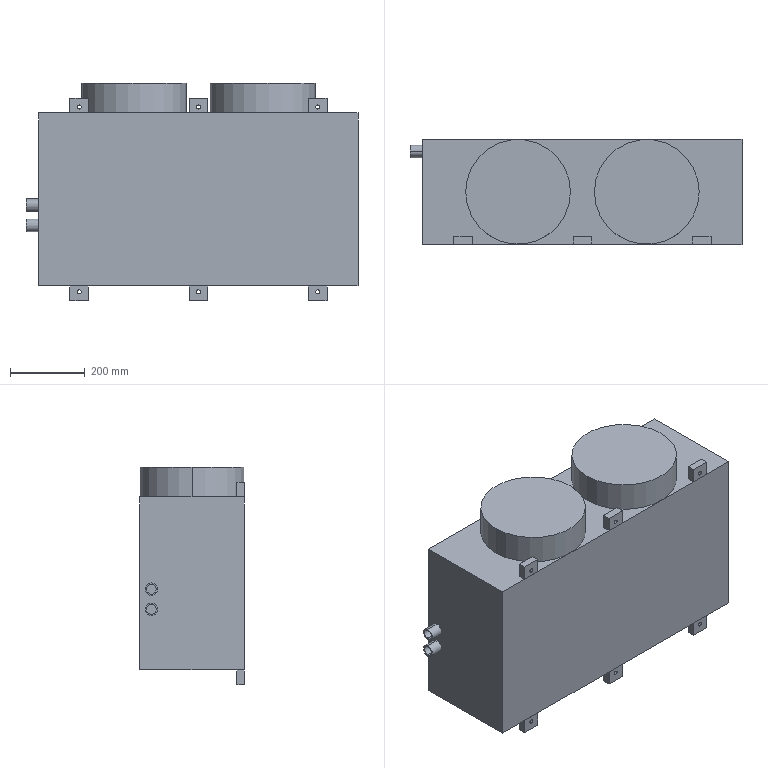Part | SolidWorks | 11 solids | 74 faces | box 890.5 x 281 x 584 mm | volume 121782593 mm3 | plane 50 | cylinder 24 | commonest cylinder face diameters 11 x12 26.5 x4 33.5 x4 281 x4